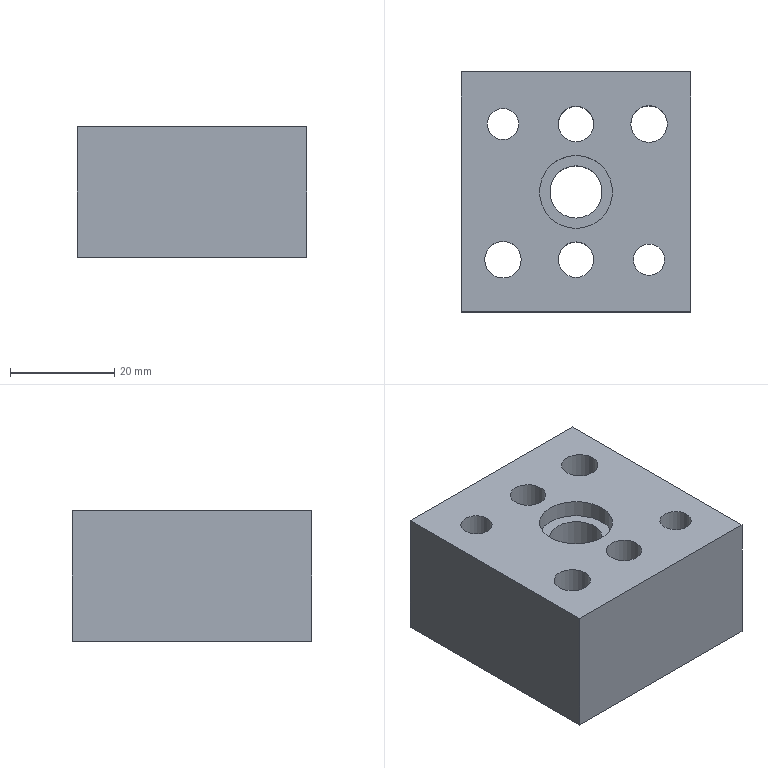Part | NX | features solid 2 | 1 solid | 23 faces | box 44 x 46 x 25 mm | volume 42055 mm3 | cylinder 12 | plane 11 | commonest cylinder face diameters 6.8 x4 6.001 x2 7 x2 11 x2 10 x1 14 x1
STEP:
#1=CARTESIAN_POINT('',(599.4,13.,10.));
#2=VERTEX_POINT('',#1);
#3=CARTESIAN_POINT('',(596.,13.,10.));
#4=DIRECTION('',(0.,0.,1.));
#5=DIRECTION('',(1.,0.,0.));
#6=AXIS2_PLACEMENT_3D('',#3,#4,#5);
#7=CIRCLE('',#6,3.4);
#8=EDGE_CURVE('',#2,#2,#7,.T.);
#9=ORIENTED_EDGE('',*,*,#8,.T.);
#10=EDGE_LOOP('',(#9));
#11=FACE_BOUND('',#10,.T.);
#12=CARTESIAN_POINT('',(592.6,13.,0.));
#13=VERTEX_POINT('',#12);
#14=CARTESIAN_POINT('',(596.,13.,0.));
#15=DIRECTION('',(0.,0.,-1.));
#16=DIRECTION('',(-1.,0.,0.));
#17=AXIS2_PLACEMENT_3D('',#14,#15,#16);
#18=CIRCLE('',#17,3.4);
#19=EDGE_CURVE('',#13,#13,#18,.T.);
#20=ORIENTED_EDGE('',*,*,#19,.T.);
#21=EDGE_LOOP('',(#20));
#22=FACE_BOUND('',#21,.T.);
#23=CARTESIAN_POINT('',(596.,13.,0.));
#24=DIRECTION('',(0.,0.,1.));
#25=DIRECTION('',(1.,0.,0.));
#26=AXIS2_PLACEMENT_3D('',#23,#24,#25);
#27=CYLINDRICAL_SURFACE('',#26,3.4);
#28=ADVANCED_FACE('',(#11,#22),#27,.F.);
#29=ORIENTED_EDGE('',*,*,#8,.F.);
#30=EDGE_LOOP('',(#29));
#31=FACE_BOUND('',#30,.T.);
#32=CARTESIAN_POINT('',(599.,13.,10.));
#33=VERTEX_POINT('',#32);
#34=CARTESIAN_POINT('',(596.,13.,10.));
#35=DIRECTION('',(0.,0.,1.));
#36=DIRECTION('',(1.,0.,0.));
#37=AXIS2_PLACEMENT_3D('',#34,#35,#36);
#38=CIRCLE('',#37,3.001);
#39=EDGE_CURVE('',#33,#33,#38,.F.);
#40=ORIENTED_EDGE('',*,*,#39,.F.);
#41=EDGE_LOOP('',(#40));
#42=FACE_BOUND('',#41,.T.);
#43=CARTESIAN_POINT('',(596.,13.,10.));
#44=DIRECTION('',(0.,0.,1.));
#45=DIRECTION('',(1.,0.,0.));
#46=AXIS2_PLACEMENT_3D('',#43,#44,#45);
#47=PLANE('',#46);
#48=ADVANCED_FACE('',(#31,#42),#47,.F.);
#49=CARTESIAN_POINT('',(627.5,13.,9.));
#50=VERTEX_POINT('',#49);
#51=CARTESIAN_POINT('',(624.,13.,9.));
#52=DIRECTION('',(0.,0.,1.));
#53=DIRECTION('',(1.,0.,0.));
#54=AXIS2_PLACEMENT_3D('',#51,#52,#53);
#55=CIRCLE('',#54,3.5);
#56=EDGE_CURVE('',#50,#50,#55,.T.);
#57=ORIENTED_EDGE('',*,*,#56,.T.);
#58=EDGE_LOOP('',(#57));
#59=FACE_BOUND('',#58,.T.);
#60=CARTESIAN_POINT('',(629.5,13.,9.));
#61=VERTEX_POINT('',#60);
#62=CARTESIAN_POINT('',(624.,13.,9.));
#63=DIRECTION('',(0.,0.,-1.));
#64=DIRECTION('',(1.,0.,0.));
#65=AXIS2_PLACEMENT_3D('',#62,#63,#64);
#66=CIRCLE('',#65,5.5);
#67=EDGE_CURVE('',#61,#61,#66,.F.);
#68=ORIENTED_EDGE('',*,*,#67,.F.);
#69=EDGE_LOOP('',(#68));
#70=FACE_BOUND('',#69,.T.);
#71=CARTESIAN_POINT('',(624.,13.,9.));
#72=DIRECTION('',(0.,0.,1.));
#73=DIRECTION('',(1.,0.,0.));
#74=AXIS2_PLACEMENT_3D('',#71,#72,#73);
#75=PLANE('',#74);
#76=ADVANCED_FACE('',(#59,#70),#75,.F.);
#77=CARTESIAN_POINT('',(610.,-5.,21.7));
#78=VERTEX_POINT('',#77);
#79=CARTESIAN_POINT('',(610.,0.,21.7));
#80=DIRECTION('',(0.,0.,-1.));
#81=DIRECTION('',(0.,-1.,0.));
#82=AXIS2_PLACEMENT_3D('',#79,#80,#81);
#83=CIRCLE('',#82,5.);
#84=EDGE_CURVE('',#78,#78,#83,.T.);
#85=ORIENTED_EDGE('',*,*,#84,.T.);
#86=EDGE_LOOP('',(#85));
#87=FACE_BOUND('',#86,.T.);
#88=CARTESIAN_POINT('',(610.,-7.,21.7));
#89=VERTEX_POINT('',#88);
#90=CARTESIAN_POINT('',(610.,0.,21.7));
#91=DIRECTION('',(0.,0.,-1.));
#92=DIRECTION('',(0.,-1.,0.));
#93=AXIS2_PLACEMENT_3D('',#90,#91,#92);
#94=CIRCLE('',#93,7.);
#95=EDGE_CURVE('',#89,#89,#94,.T.);
#96=ORIENTED_EDGE('',*,*,#95,.F.);
#97=EDGE_LOOP('',(#96));
#98=FACE_BOUND('',#97,.T.);
#99=CARTESIAN_POINT('',(610.,0.,21.7));
#100=DIRECTION('',(0.,0.,-1.));
#101=DIRECTION('',(0.,-1.,0.));
#102=AXIS2_PLACEMENT_3D('',#99,#100,#101);
#103=PLANE('',#102);
#104=ADVANCED_FACE('',(#87,#98),#103,.F.);
#105=CARTESIAN_POINT('',(599.5,-13.,9.));
#106=VERTEX_POINT('',#105);
#107=CARTESIAN_POINT('',(596.,-13.,9.));
#108=DIRECTION('',(0.,0.,1.));
#109=DIRECTION('',(1.,0.,0.));
#110=AXIS2_PLACEMENT_3D('',#107,#108,#109);
#111=CIRCLE('',#110,3.5);
#112=EDGE_CURVE('',#106,#106,#111,.T.);
#113=ORIENTED_EDGE('',*,*,#112,.T.);
#114=EDGE_LOOP('',(#113));
#115=FACE_BOUND('',#114,.T.);
#116=CARTESIAN_POINT('',(601.5,-13.,9.));
#117=VERTEX_POINT('',#116);
#118=CARTESIAN_POINT('',(596.,-13.,9.));
#119=DIRECTION('',(0.,0.,-1.));
#120=DIRECTION('',(1.,0.,0.));
#121=AXIS2_PLACEMENT_3D('',#118,#119,#120);
#122=CIRCLE('',#121,5.5);
#123=EDGE_CURVE('',#117,#117,#122,.F.);
#124=ORIENTED_EDGE('',*,*,#123,.F.);
#125=EDGE_LOOP('',(#124));
#126=FACE_BOUND('',#125,.T.);
#127=CARTESIAN_POINT('',(596.,-13.,9.));
#128=DIRECTION('',(0.,0.,1.));
#129=DIRECTION('',(1.,0.,0.));
#130=AXIS2_PLACEMENT_3D('',#127,#128,#129);
#131=PLANE('',#130);
#132=ADVANCED_FACE('',(#115,#126),#131,.F.);
#133=CARTESIAN_POINT('',(627.4,-13.,10.));
#134=VERTEX_POINT('',#133);
#135=CARTESIAN_POINT('',(624.,-13.,10.));
#136=DIRECTION('',(0.,0.,1.));
#137=DIRECTION('',(1.,0.,0.));
#138=AXIS2_PLACEMENT_3D('',#135,#136,#137);
#139=CIRCLE('',#138,3.4);
#140=EDGE_CURVE('',#134,#134,#139,.T.);
#141=ORIENTED_EDGE('',*,*,#140,.F.);
#142=EDGE_LOOP('',(#141));
#143=FACE_BOUND('',#142,.T.);
#144=CARTESIAN_POINT('',(627.,-13.,10.));
#145=VERTEX_POINT('',#144);
#146=CARTESIAN_POINT('',(624.,-13.,10.));
#147=DIRECTION('',(0.,0.,1.));
#148=DIRECTION('',(1.,0.,0.));
#149=AXIS2_PLACEMENT_3D('',#146,#147,#148);
#150=CIRCLE('',#149,3.001);
#151=EDGE_CURVE('',#145,#145,#150,.F.);
#152=ORIENTED_EDGE('',*,*,#151,.F.);
#153=EDGE_LOOP('',(#152));
#154=FACE_BOUND('',#153,.T.);
#155=CARTESIAN_POINT('',(624.,-13.,10.));
#156=DIRECTION('',(0.,0.,1.));
#157=DIRECTION('',(1.,0.,0.));
#158=AXIS2_PLACEMENT_3D('',#155,#156,#157);
#159=PLANE('',#158);
#160=ADVANCED_FACE('',(#143,#154),#159,.F.);
#161=CARTESIAN_POINT('',(610.,7.,25.));
#162=VERTEX_POINT('',#161);
#163=CARTESIAN_POINT('',(610.,0.,25.));
#164=DIRECTION('',(0.,0.,1.));
#165=DIRECTION('',(0.,1.,0.));
#166=AXIS2_PLACEMENT_3D('',#163,#164,#165);
#167=CIRCLE('',#166,7.);
#168=EDGE_CURVE('',#162,#162,#167,.T.);
#169=ORIENTED_EDGE('',*,*,#168,.T.);
#170=EDGE_LOOP('',(#169));
#171=FACE_BOUND('',#170,.T.);
#172=ORIENTED_EDGE('',*,*,#95,.T.);
#173=EDGE_LOOP('',(#172));
#174=FACE_BOUND('',#173,.T.);
#175=CARTESIAN_POINT('',(610.,0.,61.7));
#176=DIRECTION('',(0.,0.,-1.));
#177=DIRECTION('',(0.,-1.,0.));
#178=AXIS2_PLACEMENT_3D('',#175,#176,#177);
#179=CYLINDRICAL_SURFACE('',#178,7.);
#180=ADVANCED_FACE('',(#171,#174),#179,.F.);
#181=ORIENTED_EDGE('',*,*,#67,.T.);
#182=EDGE_LOOP('',(#181));
#183=FACE_BOUND('',#182,.T.);
#184=CARTESIAN_POINT('',(629.5,13.,0.));
#185=VERTEX_POINT('',#184);
#186=CARTESIAN_POINT('',(624.,13.,0.));
#187=DIRECTION('',(0.,0.,1.));
#188=DIRECTION('',(1.,0.,0.));
#189=AXIS2_PLACEMENT_3D('',#186,#187,#188);
#190=CIRCLE('',#189,5.5);
#191=EDGE_CURVE('',#185,#185,#190,.T.);
#192=ORIENTED_EDGE('',*,*,#191,.F.);
#193=EDGE_LOOP('',(#192));
#194=FACE_BOUND('',#193,.T.);
#195=CARTESIAN_POINT('',(624.,13.,0.));
#196=DIRECTION('',(0.,0.,1.));
#197=DIRECTION('',(1.,0.,0.));
#198=AXIS2_PLACEMENT_3D('',#195,#196,#197);
#199=CYLINDRICAL_SURFACE('',#198,5.5);
#200=ADVANCED_FACE('',(#183,#194),#199,.F.);
#201=CARTESIAN_POINT('',(610.,-9.6,0.));
#202=VERTEX_POINT('',#201);
#203=CARTESIAN_POINT('',(610.,-13.,0.));
#204=DIRECTION('',(0.,0.,1.));
#205=DIRECTION('',(0.,1.,0.));
#206=AXIS2_PLACEMENT_3D('',#203,#204,#205);
#207=CIRCLE('',#206,3.4);
#208=EDGE_CURVE('',#202,#202,#207,.T.);
#209=ORIENTED_EDGE('',*,*,#208,.F.);
#210=EDGE_LOOP('',(#209));
#211=FACE_BOUND('',#210,.T.);
#212=CARTESIAN_POINT('',(610.,-9.6,25.));
#213=VERTEX_POINT('',#212);
#214=CARTESIAN_POINT('',(610.,-13.,25.));
#215=DIRECTION('',(0.,0.,1.));
#216=DIRECTION('',(0.,1.,0.));
#217=AXIS2_PLACEMENT_3D('',#214,#215,#216);
#218=CIRCLE('',#217,3.4);
#219=EDGE_CURVE('',#213,#213,#218,.T.);
#220=ORIENTED_EDGE('',*,*,#219,.T.);
#221=EDGE_LOOP('',(#220));
#222=FACE_BOUND('',#221,.T.);
#223=CARTESIAN_POINT('',(610.,-13.,40.));
#224=DIRECTION('',(0.,0.,-1.));
#225=DIRECTION('',(0.,-1.,0.));
#226=AXIS2_PLACEMENT_3D('',#223,#224,#225);
#227=CYLINDRICAL_SURFACE('',#226,3.4);
#228=ADVANCED_FACE('',(#211,#222),#227,.F.);
#229=ORIENTED_EDGE('',*,*,#84,.F.);
#230=EDGE_LOOP('',(#229));
#231=FACE_BOUND('',#230,.T.);
#232=CARTESIAN_POINT('',(610.,-5.,0.));
#233=VERTEX_POINT('',#232);
#234=CARTESIAN_POINT('',(610.,0.,0.));
#235=DIRECTION('',(0.,0.,-1.));
#236=DIRECTION('',(0.,-1.,0.));
#237=AXIS2_PLACEMENT_3D('',#234,#235,#236);
#238=CIRCLE('',#237,5.);
#239=EDGE_CURVE('',#233,#233,#238,.T.);
#240=ORIENTED_EDGE('',*,*,#239,.T.);
#241=EDGE_LOOP('',(#240));
#242=FACE_BOUND('',#241,.T.);
#243=CARTESIAN_POINT('',(610.,0.,40.));
#244=DIRECTION('',(0.,0.,-1.));
#245=DIRECTION('',(0.,-1.,0.));
#246=AXIS2_PLACEMENT_3D('',#243,#244,#245);
#247=CYLINDRICAL_SURFACE('',#246,5.);
#248=ADVANCED_FACE('',(#231,#242),#247,.F.);
#249=CARTESIAN_POINT('',(588.,23.,0.));
#250=VERTEX_POINT('',#249);
#251=CARTESIAN_POINT('',(588.,23.,25.));
#252=VERTEX_POINT('',#251);
#253=CARTESIAN_POINT('',(588.,23.,-5.));
#254=DIRECTION('',(0.,0.,1.));
#255=VECTOR('',#254,1000.);
#256=LINE('',#253,#255);
#257=EDGE_CURVE('',#250,#252,#256,.T.);
#258=ORIENTED_EDGE('',*,*,#257,.F.);
#259=CARTESIAN_POINT('',(588.,-23.,0.));
#260=VERTEX_POINT('',#259);
#261=CARTESIAN_POINT('',(588.,0.,0.));
#262=DIRECTION('',(0.,1.,0.));
#263=VECTOR('',#262,1000.);
#264=LINE('',#261,#263);
#265=EDGE_CURVE('',#260,#250,#264,.T.);
#266=ORIENTED_EDGE('',*,*,#265,.F.);
#267=CARTESIAN_POINT('',(588.,-23.,25.));
#268=VERTEX_POINT('',#267);
#269=CARTESIAN_POINT('',(588.,-23.,-1.5));
#270=DIRECTION('',(0.,0.,1.));
#271=VECTOR('',#270,1000.);
#272=LINE('',#269,#271);
#273=EDGE_CURVE('',#260,#268,#272,.T.);
#274=ORIENTED_EDGE('',*,*,#273,.T.);
#275=CARTESIAN_POINT('',(588.,0.,25.));
#276=DIRECTION('',(0.,1.,0.));
#277=VECTOR('',#276,1000.);
#278=LINE('',#275,#277);
#279=EDGE_CURVE('',#252,#268,#278,.F.);
#280=ORIENTED_EDGE('',*,*,#279,.F.);
#281=EDGE_LOOP('',(#258,#266,#274,#280));
#282=FACE_BOUND('',#281,.T.);
#283=CARTESIAN_POINT('',(588.,0.,-1.5));
#284=DIRECTION('',(-1.,0.,0.));
#285=DIRECTION('',(0.,0.,1.));
#286=AXIS2_PLACEMENT_3D('',#283,#284,#285);
#287=PLANE('',#286);
#288=ADVANCED_FACE('',(#282),#287,.T.);
#289=CARTESIAN_POINT('',(632.,-23.,0.));
#290=VERTEX_POINT('',#289);
#291=CARTESIAN_POINT('',(610.,-23.,0.));
#292=DIRECTION('',(-1.,0.,0.));
#293=VECTOR('',#292,1000.);
#294=LINE('',#291,#293);
#295=EDGE_CURVE('',#290,#260,#294,.T.);
#296=ORIENTED_EDGE('',*,*,#295,.F.);
#297=CARTESIAN_POINT('',(632.,-23.,25.));
#298=VERTEX_POINT('',#297);
#299=CARTESIAN_POINT('',(632.,-23.,-5.));
#300=DIRECTION('',(0.,0.,1.));
#301=VECTOR('',#300,1000.);
#302=LINE('',#299,#301);
#303=EDGE_CURVE('',#290,#298,#302,.T.);
#304=ORIENTED_EDGE('',*,*,#303,.T.);
#305=CARTESIAN_POINT('',(610.,-23.,25.));
#306=DIRECTION('',(-1.,0.,0.));
#307=VECTOR('',#306,1000.);
#308=LINE('',#305,#307);
#309=EDGE_CURVE('',#268,#298,#308,.F.);
#310=ORIENTED_EDGE('',*,*,#309,.F.);
#311=ORIENTED_EDGE('',*,*,#273,.F.);
#312=EDGE_LOOP('',(#296,#304,#310,#311));
#313=FACE_BOUND('',#312,.T.);
#314=CARTESIAN_POINT('',(610.,-23.,-5.));
#315=DIRECTION('',(0.,-1.,0.));
#316=DIRECTION('',(0.,0.,1.));
#317=AXIS2_PLACEMENT_3D('',#314,#315,#316);
#318=PLANE('',#317);
#319=ADVANCED_FACE('',(#313),#318,.T.);
#320=CARTESIAN_POINT('',(632.,23.,25.));
#321=VERTEX_POINT('',#320);
#322=CARTESIAN_POINT('',(632.,0.,25.));
#323=DIRECTION('',(0.,1.,0.));
#324=VECTOR('',#323,1000.);
#325=LINE('',#322,#324);
#326=EDGE_CURVE('',#321,#298,#325,.F.);
#327=ORIENTED_EDGE('',*,*,#326,.T.);
#328=ORIENTED_EDGE('',*,*,#303,.F.);
#329=CARTESIAN_POINT('',(632.,23.,0.));
#330=VERTEX_POINT('',#329);
#331=CARTESIAN_POINT('',(632.,0.,0.));
#332=DIRECTION('',(0.,1.,0.));
#333=VECTOR('',#332,1000.);
#334=LINE('',#331,#333);
#335=EDGE_CURVE('',#290,#330,#334,.T.);
#336=ORIENTED_EDGE('',*,*,#335,.T.);
#337=CARTESIAN_POINT('',(632.,23.,-5.));
#338=DIRECTION('',(0.,0.,1.));
#339=VECTOR('',#338,1000.);
#340=LINE('',#337,#339);
#341=EDGE_CURVE('',#330,#321,#340,.T.);
#342=ORIENTED_EDGE('',*,*,#341,.T.);
#343=EDGE_LOOP('',(#327,#328,#336,#342));
#344=FACE_BOUND('',#343,.T.);
#345=CARTESIAN_POINT('',(632.,0.,-5.));
#346=DIRECTION('',(1.,0.,0.));
#347=DIRECTION('',(0.,0.,-1.));
#348=AXIS2_PLACEMENT_3D('',#345,#346,#347);
#349=PLANE('',#348);
#350=ADVANCED_FACE('',(#344),#349,.T.);
#351=CARTESIAN_POINT('',(610.,23.,0.));
#352=DIRECTION('',(-1.,0.,0.));
#353=VECTOR('',#352,1000.);
#354=LINE('',#351,#353);
#355=EDGE_CURVE('',#330,#250,#354,.T.);
#356=ORIENTED_EDGE('',*,*,#355,.T.);
#357=ORIENTED_EDGE('',*,*,#257,.T.);
#358=CARTESIAN_POINT('',(610.,23.,25.));
#359=DIRECTION('',(-1.,0.,0.));
#360=VECTOR('',#359,1000.);
#361=LINE('',#358,#360);
#362=EDGE_CURVE('',#252,#321,#361,.F.);
#363=ORIENTED_EDGE('',*,*,#362,.T.);
#364=ORIENTED_EDGE('',*,*,#341,.F.);
#365=EDGE_LOOP('',(#356,#357,#363,#364));
#366=FACE_BOUND('',#365,.T.);
#367=CARTESIAN_POINT('',(610.,23.,-5.));
#368=DIRECTION('',(0.,1.,0.));
#369=DIRECTION('',(0.,0.,1.));
#370=AXIS2_PLACEMENT_3D('',#367,#368,#369);
#371=PLANE('',#370);
#372=ADVANCED_FACE('',(#366),#371,.T.);
#373=CARTESIAN_POINT('',(610.,16.4,0.));
#374=VERTEX_POINT('',#373);
#375=CARTESIAN_POINT('',(610.,13.,0.));
#376=DIRECTION('',(0.,0.,1.));
#377=DIRECTION('',(0.,1.,0.));
#378=AXIS2_PLACEMENT_3D('',#375,#376,#377);
#379=CIRCLE('',#378,3.4);
#380=EDGE_CURVE('',#374,#374,#379,.T.);
#381=ORIENTED_EDGE('',*,*,#380,.F.);
#382=EDGE_LOOP('',(#381));
#383=FACE_BOUND('',#382,.T.);
#384=CARTESIAN_POINT('',(610.,16.4,25.));
#385=VERTEX_POINT('',#384);
#386=CARTESIAN_POINT('',(610.,13.,25.));
#387=DIRECTION('',(0.,0.,1.));
#388=DIRECTION('',(0.,1.,0.));
#389=AXIS2_PLACEMENT_3D('',#386,#387,#388);
#390=CIRCLE('',#389,3.4);
#391=EDGE_CURVE('',#385,#385,#390,.T.);
#392=ORIENTED_EDGE('',*,*,#391,.T.);
#393=EDGE_LOOP('',(#392));
#394=FACE_BOUND('',#393,.T.);
#395=CARTESIAN_POINT('',(610.,13.,40.));
#396=DIRECTION('',(0.,0.,-1.));
#397=DIRECTION('',(0.,-1.,0.));
#398=AXIS2_PLACEMENT_3D('',#395,#396,#397);
#399=CYLINDRICAL_SURFACE('',#398,3.4);
#400=ADVANCED_FACE('',(#383,#394),#399,.F.);
#401=ORIENTED_EDGE('',*,*,#123,.T.);
#402=EDGE_LOOP('',(#401));
#403=FACE_BOUND('',#402,.T.);
#404=CARTESIAN_POINT('',(601.5,-13.,0.));
#405=VERTEX_POINT('',#404);
#406=CARTESIAN_POINT('',(596.,-13.,0.));
#407=DIRECTION('',(0.,0.,1.));
#408=DIRECTION('',(1.,0.,0.));
#409=AXIS2_PLACEMENT_3D('',#406,#407,#408);
#410=CIRCLE('',#409,5.5);
#411=EDGE_CURVE('',#405,#405,#410,.T.);
#412=ORIENTED_EDGE('',*,*,#411,.F.);
#413=EDGE_LOOP('',(#412));
#414=FACE_BOUND('',#413,.T.);
#415=CARTESIAN_POINT('',(596.,-13.,0.));
#416=DIRECTION('',(0.,0.,1.));
#417=DIRECTION('',(1.,0.,0.));
#418=AXIS2_PLACEMENT_3D('',#415,#416,#417);
#419=CYLINDRICAL_SURFACE('',#418,5.5);
#420=ADVANCED_FACE('',(#403,#414),#419,.F.);
#421=ORIENTED_EDGE('',*,*,#140,.T.);
#422=EDGE_LOOP('',(#421));
#423=FACE_BOUND('',#422,.T.);
#424=CARTESIAN_POINT('',(627.4,-13.,0.));
#425=VERTEX_POINT('',#424);
#426=CARTESIAN_POINT('',(624.,-13.,0.));
#427=DIRECTION('',(0.,0.,1.));
#428=DIRECTION('',(1.,0.,0.));
#429=AXIS2_PLACEMENT_3D('',#426,#427,#428);
#430=CIRCLE('',#429,3.4);
#431=EDGE_CURVE('',#425,#425,#430,.T.);
#432=ORIENTED_EDGE('',*,*,#431,.F.);
#433=EDGE_LOOP('',(#432));
#434=FACE_BOUND('',#433,.T.);
#435=CARTESIAN_POINT('',(624.,-13.,0.));
#436=DIRECTION('',(0.,0.,1.));
#437=DIRECTION('',(1.,0.,0.));
#438=AXIS2_PLACEMENT_3D('',#435,#436,#437);
#439=CYLINDRICAL_SURFACE('',#438,3.4);
#440=ADVANCED_FACE('',(#423,#434),#439,.F.);
#441=ORIENTED_EDGE('',*,*,#19,.F.);
#442=EDGE_LOOP('',(#441));
#443=FACE_BOUND('',#442,.T.);
#444=ORIENTED_EDGE('',*,*,#431,.T.);
#445=EDGE_LOOP('',(#444));
#446=FACE_BOUND('',#445,.T.);
#447=ORIENTED_EDGE('',*,*,#411,.T.);
#448=EDGE_LOOP('',(#447));
#449=FACE_BOUND('',#448,.T.);
#450=ORIENTED_EDGE('',*,*,#380,.T.);
#451=EDGE_LOOP('',(#450));
#452=FACE_BOUND('',#451,.T.);
#453=ORIENTED_EDGE('',*,*,#355,.F.);
#454=ORIENTED_EDGE('',*,*,#335,.F.);
#455=ORIENTED_EDGE('',*,*,#295,.T.);
#456=ORIENTED_EDGE('',*,*,#265,.T.);
#457=EDGE_LOOP('',(#453,#454,#455,#456));
#458=FACE_BOUND('',#457,.T.);
#459=ORIENTED_EDGE('',*,*,#239,.F.);
#460=EDGE_LOOP('',(#459));
#461=FACE_BOUND('',#460,.T.);
#462=ORIENTED_EDGE('',*,*,#208,.T.);
#463=EDGE_LOOP('',(#462));
#464=FACE_BOUND('',#463,.T.);
#465=ORIENTED_EDGE('',*,*,#191,.T.);
#466=EDGE_LOOP('',(#465));
#467=FACE_BOUND('',#466,.T.);
#468=CARTESIAN_POINT('',(610.,0.,0.));
#469=DIRECTION('',(0.,0.,-1.));
#470=DIRECTION('',(-1.,0.,0.));
#471=AXIS2_PLACEMENT_3D('',#468,#469,#470);
#472=PLANE('',#471);
#473=ADVANCED_FACE('',(#443,#446,#449,#452,#458,#461,#464,#467),#472,.T.);
#474=CARTESIAN_POINT('',(592.5,-13.,25.));
#475=VERTEX_POINT('',#474);
#476=CARTESIAN_POINT('',(596.,-13.,25.));
#477=DIRECTION('',(0.,0.,-1.));
#478=DIRECTION('',(-1.,0.,0.));
#479=AXIS2_PLACEMENT_3D('',#476,#477,#478);
#480=CIRCLE('',#479,3.5);
#481=EDGE_CURVE('',#475,#475,#480,.F.);
#482=ORIENTED_EDGE('',*,*,#481,.T.);
#483=EDGE_LOOP('',(#482));
#484=FACE_BOUND('',#483,.T.);
#485=ORIENTED_EDGE('',*,*,#112,.F.);
#486=EDGE_LOOP('',(#485));
#487=FACE_BOUND('',#486,.T.);
#488=CARTESIAN_POINT('',(596.,-13.,-5.));
#489=DIRECTION('',(0.,0.,1.));
#490=DIRECTION('',(1.,0.,0.));
#491=AXIS2_PLACEMENT_3D('',#488,#489,#490);
#492=CYLINDRICAL_SURFACE('',#491,3.5);
#493=ADVANCED_FACE('',(#484,#487),#492,.F.);
#494=ORIENTED_EDGE('',*,*,#151,.T.);
#495=EDGE_LOOP('',(#494));
#496=FACE_BOUND('',#495,.T.);
#497=CARTESIAN_POINT('',(621.,-13.,25.));
#498=VERTEX_POINT('',#497);
#499=CARTESIAN_POINT('',(624.,-13.,25.));
#500=DIRECTION('',(0.,0.,-1.));
#501=DIRECTION('',(-1.,0.,0.));
#502=AXIS2_PLACEMENT_3D('',#499,#500,#501);
#503=CIRCLE('',#502,3.001);
#504=EDGE_CURVE('',#498,#498,#503,.F.);
#505=ORIENTED_EDGE('',*,*,#504,.T.);
#506=EDGE_LOOP('',(#505));
#507=FACE_BOUND('',#506,.T.);
#508=CARTESIAN_POINT('',(624.,-13.,-5.));
#509=DIRECTION('',(0.,0.,1.));
#510=DIRECTION('',(1.,0.,0.));
#511=AXIS2_PLACEMENT_3D('',#508,#509,#510);
#512=CYLINDRICAL_SURFACE('',#511,3.001);
#513=ADVANCED_FACE('',(#496,#507),#512,.F.);
#514=CARTESIAN_POINT('',(620.5,13.,25.));
#515=VERTEX_POINT('',#514);
#516=CARTESIAN_POINT('',(624.,13.,25.));
#517=DIRECTION('',(0.,0.,-1.));
#518=DIRECTION('',(-1.,0.,0.));
#519=AXIS2_PLACEMENT_3D('',#516,#517,#518);
#520=CIRCLE('',#519,3.5);
#521=EDGE_CURVE('',#515,#515,#520,.F.);
#522=ORIENTED_EDGE('',*,*,#521,.T.);
#523=EDGE_LOOP('',(#522));
#524=FACE_BOUND('',#523,.T.);
#525=ORIENTED_EDGE('',*,*,#56,.F.);
#526=EDGE_LOOP('',(#525));
#527=FACE_BOUND('',#526,.T.);
#528=CARTESIAN_POINT('',(624.,13.,-5.));
#529=DIRECTION('',(0.,0.,1.));
#530=DIRECTION('',(1.,0.,0.));
#531=AXIS2_PLACEMENT_3D('',#528,#529,#530);
#532=CYLINDRICAL_SURFACE('',#531,3.5);
#533=ADVANCED_FACE('',(#524,#527),#532,.F.);
#534=ORIENTED_EDGE('',*,*,#521,.F.);
#535=EDGE_LOOP('',(#534));
#536=FACE_BOUND('',#535,.T.);
#537=ORIENTED_EDGE('',*,*,#504,.F.);
#538=EDGE_LOOP('',(#537));
#539=FACE_BOUND('',#538,.T.);
#540=ORIENTED_EDGE('',*,*,#481,.F.);
#541=EDGE_LOOP('',(#540));
#542=FACE_BOUND('',#541,.T.);
#543=CARTESIAN_POINT('',(593.,13.,25.));
#544=VERTEX_POINT('',#543);
#545=CARTESIAN_POINT('',(596.,13.,25.));
#546=DIRECTION('',(0.,0.,-1.));
#547=DIRECTION('',(-1.,0.,0.));
#548=AXIS2_PLACEMENT_3D('',#545,#546,#547);
#549=CIRCLE('',#548,3.001);
#550=EDGE_CURVE('',#544,#544,#549,.F.);
#551=ORIENTED_EDGE('',*,*,#550,.F.);
#552=EDGE_LOOP('',(#551));
#553=FACE_BOUND('',#552,.T.);
#554=ORIENTED_EDGE('',*,*,#219,.F.);
#555=EDGE_LOOP('',(#554));
#556=FACE_BOUND('',#555,.T.);
#557=ORIENTED_EDGE('',*,*,#279,.T.);
#558=ORIENTED_EDGE('',*,*,#309,.T.);
#559=ORIENTED_EDGE('',*,*,#326,.F.);
#560=ORIENTED_EDGE('',*,*,#362,.F.);
#561=EDGE_LOOP('',(#557,#558,#559,#560));
#562=FACE_BOUND('',#561,.T.);
#563=ORIENTED_EDGE('',*,*,#391,.F.);
#564=EDGE_LOOP('',(#563));
#565=FACE_BOUND('',#564,.T.);
#566=ORIENTED_EDGE('',*,*,#168,.F.);
#567=EDGE_LOOP('',(#566));
#568=FACE_BOUND('',#567,.T.);
#569=CARTESIAN_POINT('',(512.,0.,25.));
#570=DIRECTION('',(0.,0.,-1.));
#571=DIRECTION('',(-1.,0.,0.));
#572=AXIS2_PLACEMENT_3D('',#569,#570,#571);
#573=PLANE('',#572);
#574=ADVANCED_FACE('',(#536,#539,#542,#553,#556,#562,#565,#568),#573,.F.);
#575=ORIENTED_EDGE('',*,*,#39,.T.);
#576=EDGE_LOOP('',(#575));
#577=FACE_BOUND('',#576,.T.);
#578=ORIENTED_EDGE('',*,*,#550,.T.);
#579=EDGE_LOOP('',(#578));
#580=FACE_BOUND('',#579,.T.);
#581=CARTESIAN_POINT('',(596.,13.,-5.));
#582=DIRECTION('',(0.,0.,1.));
#583=DIRECTION('',(1.,0.,0.));
#584=AXIS2_PLACEMENT_3D('',#581,#582,#583);
#585=CYLINDRICAL_SURFACE('',#584,3.001);
#586=ADVANCED_FACE('',(#577,#580),#585,.F.);
#587=CLOSED_SHELL('',(#28,#48,#76,#104,#132,#160,#180,#200,#228,#248,#288,#319,#350,#372,#400,#420,#440,#473,#493,#513,#533,#574,#586));
#588=MANIFOLD_SOLID_BREP('',#587);
#589=(LENGTH_UNIT()NAMED_UNIT(*)SI_UNIT(.MILLI.,.METRE.));
#590=UNCERTAINTY_MEASURE_WITH_UNIT(LENGTH_MEASURE(0.00001),#589,'','');
#591=(NAMED_UNIT(*)PLANE_ANGLE_UNIT()SI_UNIT($,.RADIAN.));
#592=(NAMED_UNIT(*)SI_UNIT($,.STERADIAN.)SOLID_ANGLE_UNIT());
#593=(GEOMETRIC_REPRESENTATION_CONTEXT(3)GLOBAL_UNCERTAINTY_ASSIGNED_CONTEXT((#590))GLOBAL_UNIT_ASSIGNED_CONTEXT((#589,#591,#592))REPRESENTATION_CONTEXT('',''));
#594=ADVANCED_BREP_SHAPE_REPRESENTATION('',(#588),#593);